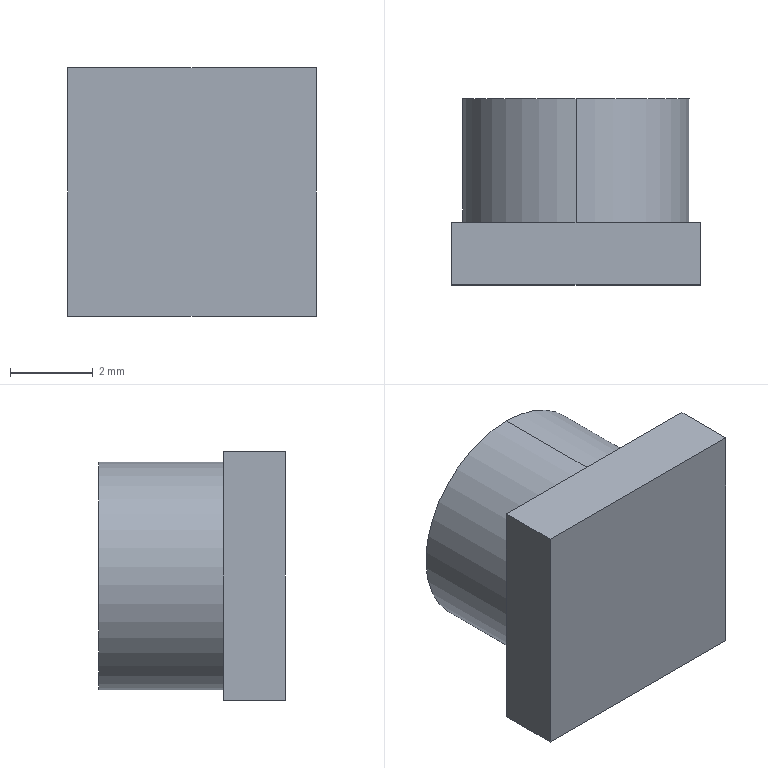Part | SolidWorks | features Extrusion 1, ICE 1 | 1 solid | 9 faces | box 6 x 4.5 x 6 mm | volume 125.275 mm3 | plane 7 | cylinder 2 | commonest cylinder face diameters 5.5 x2
STEP:
#1=CARTESIAN_POINT('',(0.,3.,2.75));
#2=VERTEX_POINT('',#1);
#3=CARTESIAN_POINT('',(0.,3.,-2.75));
#4=VERTEX_POINT('',#3);
#5=CARTESIAN_POINT('',(0.,3.,0.));
#6=DIRECTION('',(0.,1.,0.));
#7=DIRECTION('',(0.,0.,1.));
#8=AXIS2_PLACEMENT_3D('',#5,#6,#7);
#9=CIRCLE('',#8,2.75);
#10=EDGE_CURVE('',#2,#4,#9,.T.);
#11=ORIENTED_EDGE('',*,*,#10,.F.);
#12=CARTESIAN_POINT('',(0.,0.,2.75));
#13=VERTEX_POINT('',#12);
#14=CARTESIAN_POINT('',(0.,3.,2.75));
#15=DIRECTION('',(0.,-1.,0.));
#16=VECTOR('',#15,1000.);
#17=LINE('',#14,#16);
#18=EDGE_CURVE('',#2,#13,#17,.T.);
#19=ORIENTED_EDGE('',*,*,#18,.T.);
#20=CARTESIAN_POINT('',(0.,0.,-2.75));
#21=VERTEX_POINT('',#20);
#22=CARTESIAN_POINT('',(0.,0.,0.));
#23=DIRECTION('',(0.,1.,0.));
#24=DIRECTION('',(0.,0.,1.));
#25=AXIS2_PLACEMENT_3D('',#22,#23,#24);
#26=CIRCLE('',#25,2.75);
#27=EDGE_CURVE('',#13,#21,#26,.T.);
#28=ORIENTED_EDGE('',*,*,#27,.T.);
#29=CARTESIAN_POINT('',(0.,3.,-2.75));
#30=DIRECTION('',(0.,-1.,0.));
#31=VECTOR('',#30,1000.);
#32=LINE('',#29,#31);
#33=EDGE_CURVE('',#4,#21,#32,.T.);
#34=ORIENTED_EDGE('',*,*,#33,.F.);
#35=EDGE_LOOP('',(#11,#19,#28,#34));
#36=FACE_OUTER_BOUND('',#35,.T.);
#37=CARTESIAN_POINT('',(0.,3.,0.));
#38=DIRECTION('',(0.,-1.,0.));
#39=DIRECTION('',(0.,0.,-1.));
#40=AXIS2_PLACEMENT_3D('',#37,#38,#39);
#41=CYLINDRICAL_SURFACE('',#40,2.75);
#42=ADVANCED_FACE('',(#36),#41,.T.);
#43=ORIENTED_EDGE('',*,*,#18,.F.);
#44=CARTESIAN_POINT('',(0.,3.,0.));
#45=DIRECTION('',(0.,1.,0.));
#46=DIRECTION('',(0.,0.,1.));
#47=AXIS2_PLACEMENT_3D('',#44,#45,#46);
#48=CIRCLE('',#47,2.75);
#49=EDGE_CURVE('',#4,#2,#48,.T.);
#50=ORIENTED_EDGE('',*,*,#49,.F.);
#51=ORIENTED_EDGE('',*,*,#33,.T.);
#52=CARTESIAN_POINT('',(0.,0.,0.));
#53=DIRECTION('',(0.,1.,0.));
#54=DIRECTION('',(0.,0.,1.));
#55=AXIS2_PLACEMENT_3D('',#52,#53,#54);
#56=CIRCLE('',#55,2.75);
#57=EDGE_CURVE('',#21,#13,#56,.T.);
#58=ORIENTED_EDGE('',*,*,#57,.T.);
#59=EDGE_LOOP('',(#43,#50,#51,#58));
#60=FACE_OUTER_BOUND('',#59,.T.);
#61=CARTESIAN_POINT('',(0.,3.,0.));
#62=DIRECTION('',(0.,-1.,0.));
#63=DIRECTION('',(0.,0.,-1.));
#64=AXIS2_PLACEMENT_3D('',#61,#62,#63);
#65=CYLINDRICAL_SURFACE('',#64,2.75);
#66=ADVANCED_FACE('',(#60),#65,.T.);
#67=ORIENTED_EDGE('',*,*,#49,.T.);
#68=ORIENTED_EDGE('',*,*,#10,.T.);
#69=EDGE_LOOP('',(#67,#68));
#70=FACE_OUTER_BOUND('',#69,.T.);
#71=CARTESIAN_POINT('',(0.,3.,0.));
#72=DIRECTION('',(0.,1.,0.));
#73=DIRECTION('',(0.,0.,1.));
#74=AXIS2_PLACEMENT_3D('',#71,#72,#73);
#75=PLANE('',#74);
#76=ADVANCED_FACE('',(#70),#75,.T.);
#77=CARTESIAN_POINT('',(3.,0.,-3.));
#78=VERTEX_POINT('',#77);
#79=CARTESIAN_POINT('',(3.,0.,3.));
#80=VERTEX_POINT('',#79);
#81=CARTESIAN_POINT('',(3.,0.,-3.));
#82=DIRECTION('',(0.,0.,1.));
#83=VECTOR('',#82,1000.);
#84=LINE('',#81,#83);
#85=EDGE_CURVE('',#78,#80,#84,.T.);
#86=ORIENTED_EDGE('',*,*,#85,.T.);
#87=CARTESIAN_POINT('',(3.,-1.5,3.));
#88=VERTEX_POINT('',#87);
#89=CARTESIAN_POINT('',(3.,-1.5,3.));
#90=DIRECTION('',(0.,1.,0.));
#91=VECTOR('',#90,1000.);
#92=LINE('',#89,#91);
#93=EDGE_CURVE('',#88,#80,#92,.T.);
#94=ORIENTED_EDGE('',*,*,#93,.F.);
#95=CARTESIAN_POINT('',(3.,-1.5,-3.));
#96=VERTEX_POINT('',#95);
#97=CARTESIAN_POINT('',(3.,-1.5,-3.));
#98=DIRECTION('',(0.,0.,1.));
#99=VECTOR('',#98,1000.);
#100=LINE('',#97,#99);
#101=EDGE_CURVE('',#96,#88,#100,.T.);
#102=ORIENTED_EDGE('',*,*,#101,.F.);
#103=CARTESIAN_POINT('',(3.,-1.5,-3.));
#104=DIRECTION('',(0.,1.,0.));
#105=VECTOR('',#104,1000.);
#106=LINE('',#103,#105);
#107=EDGE_CURVE('',#96,#78,#106,.T.);
#108=ORIENTED_EDGE('',*,*,#107,.T.);
#109=EDGE_LOOP('',(#86,#94,#102,#108));
#110=FACE_OUTER_BOUND('',#109,.T.);
#111=CARTESIAN_POINT('',(3.,-1.5,-3.));
#112=DIRECTION('',(-1.,0.,0.));
#113=DIRECTION('',(0.,0.,1.));
#114=AXIS2_PLACEMENT_3D('',#111,#112,#113);
#115=PLANE('',#114);
#116=ADVANCED_FACE('',(#110),#115,.F.);
#117=CARTESIAN_POINT('',(-3.,0.,3.));
#118=VERTEX_POINT('',#117);
#119=CARTESIAN_POINT('',(-3.,0.,3.));
#120=DIRECTION('',(-1.,0.,0.));
#121=VECTOR('',#120,1000.);
#122=LINE('',#119,#121);
#123=EDGE_CURVE('',#80,#118,#122,.T.);
#124=ORIENTED_EDGE('',*,*,#123,.T.);
#125=CARTESIAN_POINT('',(-3.,-1.5,3.));
#126=VERTEX_POINT('',#125);
#127=CARTESIAN_POINT('',(-3.,-1.5,3.));
#128=DIRECTION('',(0.,1.,0.));
#129=VECTOR('',#128,1000.);
#130=LINE('',#127,#129);
#131=EDGE_CURVE('',#126,#118,#130,.T.);
#132=ORIENTED_EDGE('',*,*,#131,.F.);
#133=CARTESIAN_POINT('',(-3.,-1.5,3.));
#134=DIRECTION('',(-1.,0.,0.));
#135=VECTOR('',#134,1000.);
#136=LINE('',#133,#135);
#137=EDGE_CURVE('',#88,#126,#136,.T.);
#138=ORIENTED_EDGE('',*,*,#137,.F.);
#139=ORIENTED_EDGE('',*,*,#93,.T.);
#140=EDGE_LOOP('',(#124,#132,#138,#139));
#141=FACE_OUTER_BOUND('',#140,.T.);
#142=CARTESIAN_POINT('',(-3.,-1.5,3.));
#143=DIRECTION('',(0.,0.,-1.));
#144=DIRECTION('',(-1.,0.,0.));
#145=AXIS2_PLACEMENT_3D('',#142,#143,#144);
#146=PLANE('',#145);
#147=ADVANCED_FACE('',(#141),#146,.F.);
#148=CARTESIAN_POINT('',(-3.,0.,-3.));
#149=VERTEX_POINT('',#148);
#150=CARTESIAN_POINT('',(-3.,0.,-3.));
#151=DIRECTION('',(0.,0.,-1.));
#152=VECTOR('',#151,1000.);
#153=LINE('',#150,#152);
#154=EDGE_CURVE('',#118,#149,#153,.T.);
#155=ORIENTED_EDGE('',*,*,#154,.T.);
#156=CARTESIAN_POINT('',(-3.,-1.5,-3.));
#157=VERTEX_POINT('',#156);
#158=CARTESIAN_POINT('',(-3.,-1.5,-3.));
#159=DIRECTION('',(0.,1.,0.));
#160=VECTOR('',#159,1000.);
#161=LINE('',#158,#160);
#162=EDGE_CURVE('',#157,#149,#161,.T.);
#163=ORIENTED_EDGE('',*,*,#162,.F.);
#164=CARTESIAN_POINT('',(-3.,-1.5,-3.));
#165=DIRECTION('',(0.,0.,-1.));
#166=VECTOR('',#165,1000.);
#167=LINE('',#164,#166);
#168=EDGE_CURVE('',#126,#157,#167,.T.);
#169=ORIENTED_EDGE('',*,*,#168,.F.);
#170=ORIENTED_EDGE('',*,*,#131,.T.);
#171=EDGE_LOOP('',(#155,#163,#169,#170));
#172=FACE_OUTER_BOUND('',#171,.T.);
#173=CARTESIAN_POINT('',(-3.,-1.5,-3.));
#174=DIRECTION('',(1.,0.,0.));
#175=DIRECTION('',(0.,0.,-1.));
#176=AXIS2_PLACEMENT_3D('',#173,#174,#175);
#177=PLANE('',#176);
#178=ADVANCED_FACE('',(#172),#177,.F.);
#179=CARTESIAN_POINT('',(-3.,0.,-3.));
#180=DIRECTION('',(1.,0.,0.));
#181=VECTOR('',#180,1000.);
#182=LINE('',#179,#181);
#183=EDGE_CURVE('',#149,#78,#182,.T.);
#184=ORIENTED_EDGE('',*,*,#183,.T.);
#185=ORIENTED_EDGE('',*,*,#107,.F.);
#186=CARTESIAN_POINT('',(-3.,-1.5,-3.));
#187=DIRECTION('',(1.,0.,0.));
#188=VECTOR('',#187,1000.);
#189=LINE('',#186,#188);
#190=EDGE_CURVE('',#157,#96,#189,.T.);
#191=ORIENTED_EDGE('',*,*,#190,.F.);
#192=ORIENTED_EDGE('',*,*,#162,.T.);
#193=EDGE_LOOP('',(#184,#185,#191,#192));
#194=FACE_OUTER_BOUND('',#193,.T.);
#195=CARTESIAN_POINT('',(-3.,-1.5,-3.));
#196=DIRECTION('',(0.,0.,1.));
#197=DIRECTION('',(1.,0.,0.));
#198=AXIS2_PLACEMENT_3D('',#195,#196,#197);
#199=PLANE('',#198);
#200=ADVANCED_FACE('',(#194),#199,.F.);
#201=ORIENTED_EDGE('',*,*,#101,.T.);
#202=ORIENTED_EDGE('',*,*,#137,.T.);
#203=ORIENTED_EDGE('',*,*,#168,.T.);
#204=ORIENTED_EDGE('',*,*,#190,.T.);
#205=EDGE_LOOP('',(#201,#202,#203,#204));
#206=FACE_OUTER_BOUND('',#205,.T.);
#207=CARTESIAN_POINT('',(0.,-1.5,0.));
#208=DIRECTION('',(0.,1.,0.));
#209=DIRECTION('',(0.,0.,1.));
#210=AXIS2_PLACEMENT_3D('',#207,#208,#209);
#211=PLANE('',#210);
#212=ADVANCED_FACE('',(#206),#211,.F.);
#213=ORIENTED_EDGE('',*,*,#57,.F.);
#214=ORIENTED_EDGE('',*,*,#27,.F.);
#215=EDGE_LOOP('',(#213,#214));
#216=FACE_BOUND('',#215,.T.);
#217=ORIENTED_EDGE('',*,*,#85,.F.);
#218=ORIENTED_EDGE('',*,*,#183,.F.);
#219=ORIENTED_EDGE('',*,*,#154,.F.);
#220=ORIENTED_EDGE('',*,*,#123,.F.);
#221=EDGE_LOOP('',(#217,#218,#219,#220));
#222=FACE_OUTER_BOUND('',#221,.T.);
#223=CARTESIAN_POINT('',(0.,0.,0.));
#224=DIRECTION('',(0.,1.,0.));
#225=DIRECTION('',(0.,0.,1.));
#226=AXIS2_PLACEMENT_3D('',#223,#224,#225);
#227=PLANE('',#226);
#228=ADVANCED_FACE('',(#216,#222),#227,.T.);
#229=CLOSED_SHELL('',(#42,#66,#76,#116,#147,#178,#200,#212,#228));
#230=MANIFOLD_SOLID_BREP('',#229);
#231=CARTESIAN_POINT('',(0.,0.,0.));
#232=DIRECTION('',(0.,0.,1.));
#233=DIRECTION('',(1.,0.,0.));
#234=AXIS2_PLACEMENT_3D('',#231,#232,#233);
#235=(LENGTH_UNIT()NAMED_UNIT(*)SI_UNIT(.MILLI.,.METRE.));
#236=UNCERTAINTY_MEASURE_WITH_UNIT(LENGTH_MEASURE(0.00001),#235,'','');
#237=(NAMED_UNIT(*)PLANE_ANGLE_UNIT()SI_UNIT($,.RADIAN.));
#238=(NAMED_UNIT(*)SI_UNIT($,.STERADIAN.)SOLID_ANGLE_UNIT());
#239=(GEOMETRIC_REPRESENTATION_CONTEXT(3)GLOBAL_UNCERTAINTY_ASSIGNED_CONTEXT((#236))GLOBAL_UNIT_ASSIGNED_CONTEXT((#235,#237,#238))REPRESENTATION_CONTEXT('',''));
#240=ADVANCED_BREP_SHAPE_REPRESENTATION('',(#230,#234),#239);